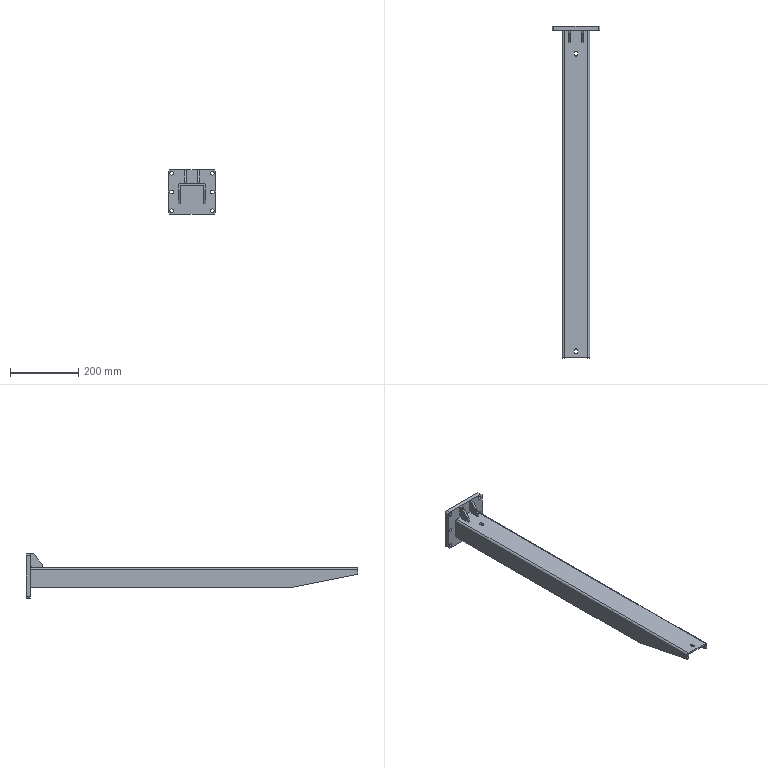Part | SolidWorks | features BaseBody 3 | 3 solids | 65 faces | box 140 x 974 x 130 mm | volume 1080338 mm3 | plane 45 | cylinder 20 | commonest cylinder face diameters 11 x12 9 x4 1.473 x2 11.473 x2